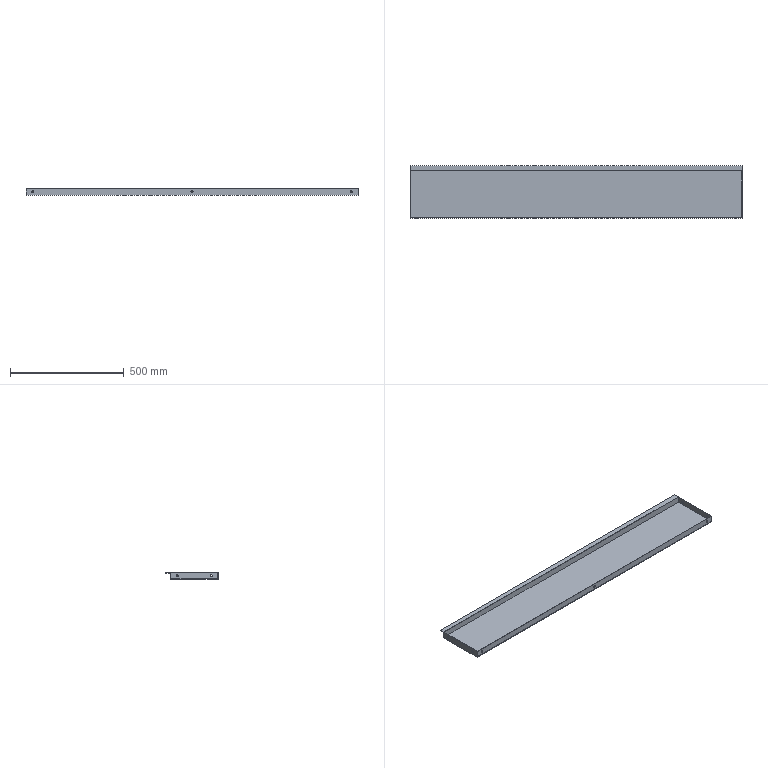Part | SolidWorks | features ICE 3, Extrusion 1, Shell 1 | 1 solid | 27 faces | box 1457 x 230 x 30 mm | volume 855585 mm3 | cylinder 14 | plane 13 | commonest cylinder face diameters 9 x14
STEP:
#1=CARTESIAN_POINT('',(2.,180.,11.5));
#2=VERTEX_POINT('',#1);
#3=CARTESIAN_POINT('',(2.,180.,20.5));
#4=VERTEX_POINT('',#3);
#5=CARTESIAN_POINT('',(2.,180.,16.));
#6=DIRECTION('',(-1.,0.,0.));
#7=DIRECTION('',(0.,0.,-1.));
#8=AXIS2_PLACEMENT_3D('',#5,#6,#7);
#9=CIRCLE('',#8,4.5);
#10=EDGE_CURVE('',#2,#4,#9,.T.);
#11=ORIENTED_EDGE('',*,*,#10,.F.);
#12=CARTESIAN_POINT('',(0.,180.,11.5));
#13=VERTEX_POINT('',#12);
#14=CARTESIAN_POINT('',(1527.,180.,11.5));
#15=DIRECTION('',(-1.,0.,0.));
#16=VECTOR('',#15,1000.);
#17=LINE('',#14,#16);
#18=EDGE_CURVE('',#2,#13,#17,.T.);
#19=ORIENTED_EDGE('',*,*,#18,.T.);
#20=CARTESIAN_POINT('',(0.,180.,20.5));
#21=VERTEX_POINT('',#20);
#22=CARTESIAN_POINT('',(0.,180.,16.));
#23=DIRECTION('',(-1.,0.,0.));
#24=DIRECTION('',(0.,0.,-1.));
#25=AXIS2_PLACEMENT_3D('',#22,#23,#24);
#26=CIRCLE('',#25,4.5);
#27=EDGE_CURVE('',#13,#21,#26,.T.);
#28=ORIENTED_EDGE('',*,*,#27,.T.);
#29=CARTESIAN_POINT('',(1527.,180.,20.5));
#30=DIRECTION('',(-1.,0.,0.));
#31=VECTOR('',#30,1000.);
#32=LINE('',#29,#31);
#33=EDGE_CURVE('',#4,#21,#32,.T.);
#34=ORIENTED_EDGE('',*,*,#33,.F.);
#35=EDGE_LOOP('',(#11,#19,#28,#34));
#36=FACE_OUTER_BOUND('',#35,.T.);
#37=CARTESIAN_POINT('',(1527.,180.,16.));
#38=DIRECTION('',(-1.,0.,0.));
#39=DIRECTION('',(0.,0.,1.));
#40=AXIS2_PLACEMENT_3D('',#37,#38,#39);
#41=CYLINDRICAL_SURFACE('',#40,4.5);
#42=ADVANCED_FACE('',(#36),#41,.F.);
#43=CARTESIAN_POINT('',(1457.,180.,20.5));
#44=VERTEX_POINT('',#43);
#45=CARTESIAN_POINT('',(1457.,180.,11.5));
#46=VERTEX_POINT('',#45);
#47=CARTESIAN_POINT('',(1457.,180.,16.));
#48=DIRECTION('',(1.,0.,0.));
#49=DIRECTION('',(0.,0.,1.));
#50=AXIS2_PLACEMENT_3D('',#47,#48,#49);
#51=CIRCLE('',#50,4.5);
#52=EDGE_CURVE('',#44,#46,#51,.T.);
#53=ORIENTED_EDGE('',*,*,#52,.T.);
#54=CARTESIAN_POINT('',(1455.,180.,11.5));
#55=VERTEX_POINT('',#54);
#56=CARTESIAN_POINT('',(1527.,180.,11.5));
#57=DIRECTION('',(-1.,0.,0.));
#58=VECTOR('',#57,1000.);
#59=LINE('',#56,#58);
#60=EDGE_CURVE('',#46,#55,#59,.T.);
#61=ORIENTED_EDGE('',*,*,#60,.T.);
#62=CARTESIAN_POINT('',(1455.,180.,20.5));
#63=VERTEX_POINT('',#62);
#64=CARTESIAN_POINT('',(1455.,180.,16.));
#65=DIRECTION('',(1.,0.,0.));
#66=DIRECTION('',(0.,0.,1.));
#67=AXIS2_PLACEMENT_3D('',#64,#65,#66);
#68=CIRCLE('',#67,4.5);
#69=EDGE_CURVE('',#63,#55,#68,.T.);
#70=ORIENTED_EDGE('',*,*,#69,.F.);
#71=CARTESIAN_POINT('',(1527.,180.,20.5));
#72=DIRECTION('',(-1.,0.,0.));
#73=VECTOR('',#72,1000.);
#74=LINE('',#71,#73);
#75=EDGE_CURVE('',#44,#63,#74,.T.);
#76=ORIENTED_EDGE('',*,*,#75,.F.);
#77=EDGE_LOOP('',(#53,#61,#70,#76));
#78=FACE_OUTER_BOUND('',#77,.T.);
#79=CARTESIAN_POINT('',(1527.,180.,16.));
#80=DIRECTION('',(-1.,0.,0.));
#81=DIRECTION('',(0.,0.,1.));
#82=AXIS2_PLACEMENT_3D('',#79,#80,#81);
#83=CYLINDRICAL_SURFACE('',#82,4.5);
#84=ADVANCED_FACE('',(#78),#83,.F.);
#85=CARTESIAN_POINT('',(2.,30.,11.5));
#86=VERTEX_POINT('',#85);
#87=CARTESIAN_POINT('',(2.,30.,20.5));
#88=VERTEX_POINT('',#87);
#89=CARTESIAN_POINT('',(2.,30.,16.));
#90=DIRECTION('',(-1.,0.,0.));
#91=DIRECTION('',(0.,0.,-1.));
#92=AXIS2_PLACEMENT_3D('',#89,#90,#91);
#93=CIRCLE('',#92,4.5);
#94=EDGE_CURVE('',#86,#88,#93,.T.);
#95=ORIENTED_EDGE('',*,*,#94,.F.);
#96=CARTESIAN_POINT('',(0.,30.,11.5));
#97=VERTEX_POINT('',#96);
#98=CARTESIAN_POINT('',(1527.,30.,11.5));
#99=DIRECTION('',(-1.,0.,0.));
#100=VECTOR('',#99,1000.);
#101=LINE('',#98,#100);
#102=EDGE_CURVE('',#86,#97,#101,.T.);
#103=ORIENTED_EDGE('',*,*,#102,.T.);
#104=CARTESIAN_POINT('',(0.,30.,20.5));
#105=VERTEX_POINT('',#104);
#106=CARTESIAN_POINT('',(0.,30.,16.));
#107=DIRECTION('',(-1.,0.,0.));
#108=DIRECTION('',(0.,0.,-1.));
#109=AXIS2_PLACEMENT_3D('',#106,#107,#108);
#110=CIRCLE('',#109,4.5);
#111=EDGE_CURVE('',#97,#105,#110,.T.);
#112=ORIENTED_EDGE('',*,*,#111,.T.);
#113=CARTESIAN_POINT('',(1527.,30.,20.5));
#114=DIRECTION('',(-1.,0.,0.));
#115=VECTOR('',#114,1000.);
#116=LINE('',#113,#115);
#117=EDGE_CURVE('',#88,#105,#116,.T.);
#118=ORIENTED_EDGE('',*,*,#117,.F.);
#119=EDGE_LOOP('',(#95,#103,#112,#118));
#120=FACE_OUTER_BOUND('',#119,.T.);
#121=CARTESIAN_POINT('',(1527.,30.,16.));
#122=DIRECTION('',(-1.,0.,0.));
#123=DIRECTION('',(0.,0.,1.));
#124=AXIS2_PLACEMENT_3D('',#121,#122,#123);
#125=CYLINDRICAL_SURFACE('',#124,4.5);
#126=ADVANCED_FACE('',(#120),#125,.F.);
#127=CARTESIAN_POINT('',(1457.,30.,20.5));
#128=VERTEX_POINT('',#127);
#129=CARTESIAN_POINT('',(1457.,30.,11.5));
#130=VERTEX_POINT('',#129);
#131=CARTESIAN_POINT('',(1457.,30.,16.));
#132=DIRECTION('',(1.,0.,0.));
#133=DIRECTION('',(0.,0.,1.));
#134=AXIS2_PLACEMENT_3D('',#131,#132,#133);
#135=CIRCLE('',#134,4.5);
#136=EDGE_CURVE('',#128,#130,#135,.T.);
#137=ORIENTED_EDGE('',*,*,#136,.T.);
#138=CARTESIAN_POINT('',(1455.,30.,11.5));
#139=VERTEX_POINT('',#138);
#140=CARTESIAN_POINT('',(1527.,30.,11.5));
#141=DIRECTION('',(-1.,0.,0.));
#142=VECTOR('',#141,1000.);
#143=LINE('',#140,#142);
#144=EDGE_CURVE('',#130,#139,#143,.T.);
#145=ORIENTED_EDGE('',*,*,#144,.T.);
#146=CARTESIAN_POINT('',(1455.,30.,20.5));
#147=VERTEX_POINT('',#146);
#148=CARTESIAN_POINT('',(1455.,30.,16.));
#149=DIRECTION('',(1.,0.,0.));
#150=DIRECTION('',(0.,0.,1.));
#151=AXIS2_PLACEMENT_3D('',#148,#149,#150);
#152=CIRCLE('',#151,4.5);
#153=EDGE_CURVE('',#147,#139,#152,.T.);
#154=ORIENTED_EDGE('',*,*,#153,.F.);
#155=CARTESIAN_POINT('',(1527.,30.,20.5));
#156=DIRECTION('',(-1.,0.,0.));
#157=VECTOR('',#156,1000.);
#158=LINE('',#155,#157);
#159=EDGE_CURVE('',#128,#147,#158,.T.);
#160=ORIENTED_EDGE('',*,*,#159,.F.);
#161=EDGE_LOOP('',(#137,#145,#154,#160));
#162=FACE_OUTER_BOUND('',#161,.T.);
#163=CARTESIAN_POINT('',(1527.,30.,16.));
#164=DIRECTION('',(-1.,0.,0.));
#165=DIRECTION('',(0.,0.,1.));
#166=AXIS2_PLACEMENT_3D('',#163,#164,#165);
#167=CYLINDRICAL_SURFACE('',#166,4.5);
#168=ADVANCED_FACE('',(#162),#167,.F.);
#169=CARTESIAN_POINT('',(30.,0.,11.5));
#170=VERTEX_POINT('',#169);
#171=CARTESIAN_POINT('',(30.,0.,20.5));
#172=VERTEX_POINT('',#171);
#173=CARTESIAN_POINT('',(30.,0.,16.));
#174=DIRECTION('',(0.,1.,0.));
#175=DIRECTION('',(0.,0.,1.));
#176=AXIS2_PLACEMENT_3D('',#173,#174,#175);
#177=CIRCLE('',#176,4.5);
#178=EDGE_CURVE('',#170,#172,#177,.T.);
#179=ORIENTED_EDGE('',*,*,#178,.F.);
#180=CARTESIAN_POINT('',(30.,2.,11.5));
#181=VERTEX_POINT('',#180);
#182=CARTESIAN_POINT('',(30.,-8.,11.5));
#183=DIRECTION('',(0.,1.,0.));
#184=VECTOR('',#183,1000.);
#185=LINE('',#182,#184);
#186=EDGE_CURVE('',#170,#181,#185,.T.);
#187=ORIENTED_EDGE('',*,*,#186,.T.);
#188=CARTESIAN_POINT('',(30.,2.,20.5));
#189=VERTEX_POINT('',#188);
#190=CARTESIAN_POINT('',(30.,2.,16.));
#191=DIRECTION('',(0.,1.,0.));
#192=DIRECTION('',(0.,0.,1.));
#193=AXIS2_PLACEMENT_3D('',#190,#191,#192);
#194=CIRCLE('',#193,4.5);
#195=EDGE_CURVE('',#181,#189,#194,.T.);
#196=ORIENTED_EDGE('',*,*,#195,.T.);
#197=CARTESIAN_POINT('',(30.,-8.,20.5));
#198=DIRECTION('',(0.,1.,0.));
#199=VECTOR('',#198,1000.);
#200=LINE('',#197,#199);
#201=EDGE_CURVE('',#172,#189,#200,.T.);
#202=ORIENTED_EDGE('',*,*,#201,.F.);
#203=EDGE_LOOP('',(#179,#187,#196,#202));
#204=FACE_OUTER_BOUND('',#203,.T.);
#205=CARTESIAN_POINT('',(30.,-8.,16.));
#206=DIRECTION('',(0.,1.,0.));
#207=DIRECTION('',(0.,0.,1.));
#208=AXIS2_PLACEMENT_3D('',#205,#206,#207);
#209=CYLINDRICAL_SURFACE('',#208,4.5);
#210=ADVANCED_FACE('',(#204),#209,.F.);
#211=CARTESIAN_POINT('',(728.5,0.,11.5));
#212=VERTEX_POINT('',#211);
#213=CARTESIAN_POINT('',(728.5,0.,20.5));
#214=VERTEX_POINT('',#213);
#215=CARTESIAN_POINT('',(728.5,0.,16.));
#216=DIRECTION('',(0.,1.,0.));
#217=DIRECTION('',(0.,0.,1.));
#218=AXIS2_PLACEMENT_3D('',#215,#216,#217);
#219=CIRCLE('',#218,4.5);
#220=EDGE_CURVE('',#212,#214,#219,.T.);
#221=ORIENTED_EDGE('',*,*,#220,.F.);
#222=CARTESIAN_POINT('',(728.5,2.,11.5));
#223=VERTEX_POINT('',#222);
#224=CARTESIAN_POINT('',(728.5,-8.,11.5));
#225=DIRECTION('',(0.,1.,0.));
#226=VECTOR('',#225,1000.);
#227=LINE('',#224,#226);
#228=EDGE_CURVE('',#212,#223,#227,.T.);
#229=ORIENTED_EDGE('',*,*,#228,.T.);
#230=CARTESIAN_POINT('',(728.5,2.,20.5));
#231=VERTEX_POINT('',#230);
#232=CARTESIAN_POINT('',(728.5,2.,16.));
#233=DIRECTION('',(0.,1.,0.));
#234=DIRECTION('',(0.,0.,1.));
#235=AXIS2_PLACEMENT_3D('',#232,#233,#234);
#236=CIRCLE('',#235,4.5);
#237=EDGE_CURVE('',#223,#231,#236,.T.);
#238=ORIENTED_EDGE('',*,*,#237,.T.);
#239=CARTESIAN_POINT('',(728.5,-8.,20.5));
#240=DIRECTION('',(0.,1.,0.));
#241=VECTOR('',#240,1000.);
#242=LINE('',#239,#241);
#243=EDGE_CURVE('',#214,#231,#242,.T.);
#244=ORIENTED_EDGE('',*,*,#243,.F.);
#245=EDGE_LOOP('',(#221,#229,#238,#244));
#246=FACE_OUTER_BOUND('',#245,.T.);
#247=CARTESIAN_POINT('',(728.5,-8.,16.));
#248=DIRECTION('',(0.,1.,0.));
#249=DIRECTION('',(0.,0.,1.));
#250=AXIS2_PLACEMENT_3D('',#247,#248,#249);
#251=CYLINDRICAL_SURFACE('',#250,4.5);
#252=ADVANCED_FACE('',(#246),#251,.F.);
#253=CARTESIAN_POINT('',(1427.,0.,11.5));
#254=VERTEX_POINT('',#253);
#255=CARTESIAN_POINT('',(1427.,0.,20.5));
#256=VERTEX_POINT('',#255);
#257=CARTESIAN_POINT('',(1427.,0.,16.));
#258=DIRECTION('',(0.,1.,0.));
#259=DIRECTION('',(0.,0.,1.));
#260=AXIS2_PLACEMENT_3D('',#257,#258,#259);
#261=CIRCLE('',#260,4.5);
#262=EDGE_CURVE('',#254,#256,#261,.T.);
#263=ORIENTED_EDGE('',*,*,#262,.F.);
#264=CARTESIAN_POINT('',(1427.,2.,11.5));
#265=VERTEX_POINT('',#264);
#266=CARTESIAN_POINT('',(1427.,-8.,11.5));
#267=DIRECTION('',(0.,1.,0.));
#268=VECTOR('',#267,1000.);
#269=LINE('',#266,#268);
#270=EDGE_CURVE('',#254,#265,#269,.T.);
#271=ORIENTED_EDGE('',*,*,#270,.T.);
#272=CARTESIAN_POINT('',(1427.,2.,20.5));
#273=VERTEX_POINT('',#272);
#274=CARTESIAN_POINT('',(1427.,2.,16.));
#275=DIRECTION('',(0.,1.,0.));
#276=DIRECTION('',(0.,0.,1.));
#277=AXIS2_PLACEMENT_3D('',#274,#275,#276);
#278=CIRCLE('',#277,4.5);
#279=EDGE_CURVE('',#265,#273,#278,.T.);
#280=ORIENTED_EDGE('',*,*,#279,.T.);
#281=CARTESIAN_POINT('',(1427.,-8.,20.5));
#282=DIRECTION('',(0.,1.,0.));
#283=VECTOR('',#282,1000.);
#284=LINE('',#281,#283);
#285=EDGE_CURVE('',#256,#273,#284,.T.);
#286=ORIENTED_EDGE('',*,*,#285,.F.);
#287=EDGE_LOOP('',(#263,#271,#280,#286));
#288=FACE_OUTER_BOUND('',#287,.T.);
#289=CARTESIAN_POINT('',(1427.,-8.,16.));
#290=DIRECTION('',(0.,1.,0.));
#291=DIRECTION('',(0.,0.,1.));
#292=AXIS2_PLACEMENT_3D('',#289,#290,#291);
#293=CYLINDRICAL_SURFACE('',#292,4.5);
#294=ADVANCED_FACE('',(#288),#293,.F.);
#295=CARTESIAN_POINT('',(0.,30.,16.));
#296=DIRECTION('',(-1.,0.,0.));
#297=DIRECTION('',(0.,0.,-1.));
#298=AXIS2_PLACEMENT_3D('',#295,#296,#297);
#299=CIRCLE('',#298,4.5);
#300=EDGE_CURVE('',#105,#97,#299,.T.);
#301=ORIENTED_EDGE('',*,*,#300,.F.);
#302=ORIENTED_EDGE('',*,*,#111,.F.);
#303=EDGE_LOOP('',(#301,#302));
#304=FACE_BOUND('',#303,.T.);
#305=CARTESIAN_POINT('',(0.,210.,0.));
#306=VERTEX_POINT('',#305);
#307=CARTESIAN_POINT('',(0.,0.,0.));
#308=VERTEX_POINT('',#307);
#309=CARTESIAN_POINT('',(0.,0.,0.));
#310=DIRECTION('',(0.,-1.,0.));
#311=VECTOR('',#310,1000.);
#312=LINE('',#309,#311);
#313=EDGE_CURVE('',#306,#308,#312,.T.);
#314=ORIENTED_EDGE('',*,*,#313,.T.);
#315=CARTESIAN_POINT('',(0.,0.,30.));
#316=VERTEX_POINT('',#315);
#317=CARTESIAN_POINT('',(0.,0.,30.));
#318=DIRECTION('',(0.,0.,-1.));
#319=VECTOR('',#318,1000.);
#320=LINE('',#317,#319);
#321=EDGE_CURVE('',#316,#308,#320,.T.);
#322=ORIENTED_EDGE('',*,*,#321,.F.);
#323=CARTESIAN_POINT('',(0.,230.,30.));
#324=VERTEX_POINT('',#323);
#325=CARTESIAN_POINT('',(0.,0.,30.));
#326=DIRECTION('',(0.,-1.,0.));
#327=VECTOR('',#326,1000.);
#328=LINE('',#325,#327);
#329=EDGE_CURVE('',#324,#316,#328,.T.);
#330=ORIENTED_EDGE('',*,*,#329,.F.);
#331=CARTESIAN_POINT('',(0.,230.,28.));
#332=VERTEX_POINT('',#331);
#333=CARTESIAN_POINT('',(0.,230.,28.));
#334=DIRECTION('',(0.,0.,1.));
#335=VECTOR('',#334,1000.);
#336=LINE('',#333,#335);
#337=EDGE_CURVE('',#332,#324,#336,.T.);
#338=ORIENTED_EDGE('',*,*,#337,.F.);
#339=CARTESIAN_POINT('',(0.,210.,28.));
#340=VERTEX_POINT('',#339);
#341=CARTESIAN_POINT('',(0.,230.,28.));
#342=DIRECTION('',(0.,-1.,0.));
#343=VECTOR('',#342,1000.);
#344=LINE('',#341,#343);
#345=EDGE_CURVE('',#332,#340,#344,.T.);
#346=ORIENTED_EDGE('',*,*,#345,.T.);
#347=CARTESIAN_POINT('',(0.,210.,30.));
#348=DIRECTION('',(0.,0.,-1.));
#349=VECTOR('',#348,1000.);
#350=LINE('',#347,#349);
#351=EDGE_CURVE('',#340,#306,#350,.T.);
#352=ORIENTED_EDGE('',*,*,#351,.T.);
#353=EDGE_LOOP('',(#314,#322,#330,#338,#346,#352));
#354=FACE_OUTER_BOUND('',#353,.T.);
#355=CARTESIAN_POINT('',(0.,180.,16.));
#356=DIRECTION('',(-1.,0.,0.));
#357=DIRECTION('',(0.,0.,-1.));
#358=AXIS2_PLACEMENT_3D('',#355,#356,#357);
#359=CIRCLE('',#358,4.5);
#360=EDGE_CURVE('',#21,#13,#359,.T.);
#361=ORIENTED_EDGE('',*,*,#360,.F.);
#362=ORIENTED_EDGE('',*,*,#27,.F.);
#363=EDGE_LOOP('',(#361,#362));
#364=FACE_BOUND('',#363,.T.);
#365=CARTESIAN_POINT('',(0.,0.,30.));
#366=DIRECTION('',(1.,0.,0.));
#367=DIRECTION('',(0.,0.,-1.));
#368=AXIS2_PLACEMENT_3D('',#365,#366,#367);
#369=PLANE('',#368);
#370=ADVANCED_FACE('',(#304,#354,#364),#369,.F.);
#371=ORIENTED_EDGE('',*,*,#136,.F.);
#372=CARTESIAN_POINT('',(1457.,30.,16.));
#373=DIRECTION('',(1.,0.,0.));
#374=DIRECTION('',(0.,0.,1.));
#375=AXIS2_PLACEMENT_3D('',#372,#373,#374);
#376=CIRCLE('',#375,4.5);
#377=EDGE_CURVE('',#130,#128,#376,.T.);
#378=ORIENTED_EDGE('',*,*,#377,.F.);
#379=EDGE_LOOP('',(#371,#378));
#380=FACE_BOUND('',#379,.T.);
#381=CARTESIAN_POINT('',(1457.,0.,0.));
#382=VERTEX_POINT('',#381);
#383=CARTESIAN_POINT('',(1457.,210.,0.));
#384=VERTEX_POINT('',#383);
#385=CARTESIAN_POINT('',(1457.,0.,0.));
#386=DIRECTION('',(0.,1.,0.));
#387=VECTOR('',#386,1000.);
#388=LINE('',#385,#387);
#389=EDGE_CURVE('',#382,#384,#388,.T.);
#390=ORIENTED_EDGE('',*,*,#389,.T.);
#391=CARTESIAN_POINT('',(1457.,210.,28.));
#392=VERTEX_POINT('',#391);
#393=CARTESIAN_POINT('',(1457.,210.,30.));
#394=DIRECTION('',(0.,0.,-1.));
#395=VECTOR('',#394,1000.);
#396=LINE('',#393,#395);
#397=EDGE_CURVE('',#392,#384,#396,.T.);
#398=ORIENTED_EDGE('',*,*,#397,.F.);
#399=CARTESIAN_POINT('',(1457.,230.,28.));
#400=VERTEX_POINT('',#399);
#401=CARTESIAN_POINT('',(1457.,210.,28.));
#402=DIRECTION('',(0.,1.,0.));
#403=VECTOR('',#402,1000.);
#404=LINE('',#401,#403);
#405=EDGE_CURVE('',#392,#400,#404,.T.);
#406=ORIENTED_EDGE('',*,*,#405,.T.);
#407=CARTESIAN_POINT('',(1457.,230.,30.));
#408=VERTEX_POINT('',#407);
#409=CARTESIAN_POINT('',(1457.,230.,28.));
#410=DIRECTION('',(0.,0.,1.));
#411=VECTOR('',#410,1000.);
#412=LINE('',#409,#411);
#413=EDGE_CURVE('',#400,#408,#412,.T.);
#414=ORIENTED_EDGE('',*,*,#413,.T.);
#415=CARTESIAN_POINT('',(1457.,0.,30.));
#416=VERTEX_POINT('',#415);
#417=CARTESIAN_POINT('',(1457.,0.,30.));
#418=DIRECTION('',(0.,1.,0.));
#419=VECTOR('',#418,1000.);
#420=LINE('',#417,#419);
#421=EDGE_CURVE('',#416,#408,#420,.T.);
#422=ORIENTED_EDGE('',*,*,#421,.F.);
#423=CARTESIAN_POINT('',(1457.,0.,30.));
#424=DIRECTION('',(0.,0.,-1.));
#425=VECTOR('',#424,1000.);
#426=LINE('',#423,#425);
#427=EDGE_CURVE('',#416,#382,#426,.T.);
#428=ORIENTED_EDGE('',*,*,#427,.T.);
#429=EDGE_LOOP('',(#390,#398,#406,#414,#422,#428));
#430=FACE_OUTER_BOUND('',#429,.T.);
#431=ORIENTED_EDGE('',*,*,#52,.F.);
#432=CARTESIAN_POINT('',(1457.,180.,16.));
#433=DIRECTION('',(1.,0.,0.));
#434=DIRECTION('',(0.,0.,1.));
#435=AXIS2_PLACEMENT_3D('',#432,#433,#434);
#436=CIRCLE('',#435,4.5);
#437=EDGE_CURVE('',#46,#44,#436,.T.);
#438=ORIENTED_EDGE('',*,*,#437,.F.);
#439=EDGE_LOOP('',(#431,#438));
#440=FACE_BOUND('',#439,.T.);
#441=CARTESIAN_POINT('',(1457.,0.,30.));
#442=DIRECTION('',(-1.,0.,0.));
#443=DIRECTION('',(0.,0.,1.));
#444=AXIS2_PLACEMENT_3D('',#441,#442,#443);
#445=PLANE('',#444);
#446=ADVANCED_FACE('',(#380,#430,#440),#445,.F.);
#447=CARTESIAN_POINT('',(2.,30.,16.));
#448=DIRECTION('',(-1.,0.,0.));
#449=DIRECTION('',(0.,0.,-1.));
#450=AXIS2_PLACEMENT_3D('',#447,#448,#449);
#451=CIRCLE('',#450,4.5);
#452=EDGE_CURVE('',#88,#86,#451,.T.);
#453=ORIENTED_EDGE('',*,*,#452,.T.);
#454=ORIENTED_EDGE('',*,*,#94,.T.);
#455=EDGE_LOOP('',(#453,#454));
#456=FACE_BOUND('',#455,.T.);
#457=CARTESIAN_POINT('',(2.,208.,2.));
#458=VERTEX_POINT('',#457);
#459=CARTESIAN_POINT('',(2.,2.,2.));
#460=VERTEX_POINT('',#459);
#461=CARTESIAN_POINT('',(2.,210.,2.));
#462=DIRECTION('',(0.,-1.,0.));
#463=VECTOR('',#462,1000.);
#464=LINE('',#461,#463);
#465=EDGE_CURVE('',#458,#460,#464,.T.);
#466=ORIENTED_EDGE('',*,*,#465,.F.);
#467=CARTESIAN_POINT('',(2.,208.,30.));
#468=VERTEX_POINT('',#467);
#469=CARTESIAN_POINT('',(2.,208.,30.));
#470=DIRECTION('',(0.,0.,-1.));
#471=VECTOR('',#470,1000.);
#472=LINE('',#469,#471);
#473=EDGE_CURVE('',#468,#458,#472,.T.);
#474=ORIENTED_EDGE('',*,*,#473,.F.);
#475=CARTESIAN_POINT('',(2.,2.,30.));
#476=VERTEX_POINT('',#475);
#477=CARTESIAN_POINT('',(2.,210.,30.));
#478=DIRECTION('',(0.,-1.,0.));
#479=VECTOR('',#478,1000.);
#480=LINE('',#477,#479);
#481=EDGE_CURVE('',#468,#476,#480,.T.);
#482=ORIENTED_EDGE('',*,*,#481,.T.);
#483=CARTESIAN_POINT('',(2.,2.,30.));
#484=DIRECTION('',(0.,0.,-1.));
#485=VECTOR('',#484,1000.);
#486=LINE('',#483,#485);
#487=EDGE_CURVE('',#476,#460,#486,.T.);
#488=ORIENTED_EDGE('',*,*,#487,.T.);
#489=EDGE_LOOP('',(#466,#474,#482,#488));
#490=FACE_OUTER_BOUND('',#489,.T.);
#491=CARTESIAN_POINT('',(2.,180.,16.));
#492=DIRECTION('',(-1.,0.,0.));
#493=DIRECTION('',(0.,0.,-1.));
#494=AXIS2_PLACEMENT_3D('',#491,#492,#493);
#495=CIRCLE('',#494,4.5);
#496=EDGE_CURVE('',#4,#2,#495,.T.);
#497=ORIENTED_EDGE('',*,*,#496,.T.);
#498=ORIENTED_EDGE('',*,*,#10,.T.);
#499=EDGE_LOOP('',(#497,#498));
#500=FACE_BOUND('',#499,.T.);
#501=CARTESIAN_POINT('',(2.,0.,30.));
#502=DIRECTION('',(1.,0.,0.));
#503=DIRECTION('',(0.,0.,-1.));
#504=AXIS2_PLACEMENT_3D('',#501,#502,#503);
#505=PLANE('',#504);
#506=ADVANCED_FACE('',(#456,#490,#500),#505,.T.);
#507=ORIENTED_EDGE('',*,*,#153,.T.);
#508=CARTESIAN_POINT('',(1455.,30.,16.));
#509=DIRECTION('',(1.,0.,0.));
#510=DIRECTION('',(0.,0.,1.));
#511=AXIS2_PLACEMENT_3D('',#508,#509,#510);
#512=CIRCLE('',#511,4.5);
#513=EDGE_CURVE('',#139,#147,#512,.T.);
#514=ORIENTED_EDGE('',*,*,#513,.T.);
#515=EDGE_LOOP('',(#507,#514));
#516=FACE_BOUND('',#515,.T.);
#517=CARTESIAN_POINT('',(1455.,2.,2.));
#518=VERTEX_POINT('',#517);
#519=CARTESIAN_POINT('',(1455.,208.,2.));
#520=VERTEX_POINT('',#519);
#521=CARTESIAN_POINT('',(1455.,210.,2.));
#522=DIRECTION('',(0.,1.,0.));
#523=VECTOR('',#522,1000.);
#524=LINE('',#521,#523);
#525=EDGE_CURVE('',#518,#520,#524,.T.);
#526=ORIENTED_EDGE('',*,*,#525,.F.);
#527=CARTESIAN_POINT('',(1455.,2.,30.));
#528=VERTEX_POINT('',#527);
#529=CARTESIAN_POINT('',(1455.,2.,30.));
#530=DIRECTION('',(0.,0.,-1.));
#531=VECTOR('',#530,1000.);
#532=LINE('',#529,#531);
#533=EDGE_CURVE('',#528,#518,#532,.T.);
#534=ORIENTED_EDGE('',*,*,#533,.F.);
#535=CARTESIAN_POINT('',(1455.,208.,30.));
#536=VERTEX_POINT('',#535);
#537=CARTESIAN_POINT('',(1455.,210.,30.));
#538=DIRECTION('',(0.,1.,0.));
#539=VECTOR('',#538,1000.);
#540=LINE('',#537,#539);
#541=EDGE_CURVE('',#528,#536,#540,.T.);
#542=ORIENTED_EDGE('',*,*,#541,.T.);
#543=CARTESIAN_POINT('',(1455.,208.,30.));
#544=DIRECTION('',(0.,0.,-1.));
#545=VECTOR('',#544,1000.);
#546=LINE('',#543,#545);
#547=EDGE_CURVE('',#536,#520,#546,.T.);
#548=ORIENTED_EDGE('',*,*,#547,.T.);
#549=EDGE_LOOP('',(#526,#534,#542,#548));
#550=FACE_OUTER_BOUND('',#549,.T.);
#551=ORIENTED_EDGE('',*,*,#69,.T.);
#552=CARTESIAN_POINT('',(1455.,180.,16.));
#553=DIRECTION('',(1.,0.,0.));
#554=DIRECTION('',(0.,0.,1.));
#555=AXIS2_PLACEMENT_3D('',#552,#553,#554);
#556=CIRCLE('',#555,4.5);
#557=EDGE_CURVE('',#55,#63,#556,.T.);
#558=ORIENTED_EDGE('',*,*,#557,.T.);
#559=EDGE_LOOP('',(#551,#558));
#560=FACE_BOUND('',#559,.T.);
#561=CARTESIAN_POINT('',(1455.,0.,30.));
#562=DIRECTION('',(-1.,0.,0.));
#563=DIRECTION('',(0.,0.,1.));
#564=AXIS2_PLACEMENT_3D('',#561,#562,#563);
#565=PLANE('',#564);
#566=ADVANCED_FACE('',(#516,#550,#560),#565,.T.);
#567=ORIENTED_EDGE('',*,*,#329,.T.);
#568=CARTESIAN_POINT('',(0.,0.,30.));
#569=DIRECTION('',(1.,0.,0.));
#570=VECTOR('',#569,1000.);
#571=LINE('',#568,#570);
#572=EDGE_CURVE('',#316,#416,#571,.T.);
#573=ORIENTED_EDGE('',*,*,#572,.T.);
#574=ORIENTED_EDGE('',*,*,#421,.T.);
#575=CARTESIAN_POINT('',(0.,230.,30.));
#576=DIRECTION('',(-1.,0.,0.));
#577=VECTOR('',#576,1000.);
#578=LINE('',#575,#577);
#579=EDGE_CURVE('',#408,#324,#578,.T.);
#580=ORIENTED_EDGE('',*,*,#579,.T.);
#581=EDGE_LOOP('',(#567,#573,#574,#580));
#582=FACE_OUTER_BOUND('',#581,.T.);
#583=ORIENTED_EDGE('',*,*,#481,.F.);
#584=CARTESIAN_POINT('',(0.,208.,30.));
#585=DIRECTION('',(-1.,0.,0.));
#586=VECTOR('',#585,1000.);
#587=LINE('',#584,#586);
#588=EDGE_CURVE('',#536,#468,#587,.T.);
#589=ORIENTED_EDGE('',*,*,#588,.F.);
#590=ORIENTED_EDGE('',*,*,#541,.F.);
#591=CARTESIAN_POINT('',(0.,2.,30.));
#592=DIRECTION('',(1.,0.,0.));
#593=VECTOR('',#592,1000.);
#594=LINE('',#591,#593);
#595=EDGE_CURVE('',#476,#528,#594,.T.);
#596=ORIENTED_EDGE('',*,*,#595,.F.);
#597=EDGE_LOOP('',(#583,#589,#590,#596));
#598=FACE_BOUND('',#597,.T.);
#599=CARTESIAN_POINT('',(0.,210.,30.));
#600=DIRECTION('',(0.,0.,-1.));
#601=DIRECTION('',(-1.,0.,0.));
#602=AXIS2_PLACEMENT_3D('',#599,#600,#601);
#603=PLANE('',#602);
#604=ADVANCED_FACE('',(#582,#598),#603,.F.);
#605=CARTESIAN_POINT('',(30.,0.,16.));
#606=DIRECTION('',(0.,1.,0.));
#607=DIRECTION('',(0.,0.,1.));
#608=AXIS2_PLACEMENT_3D('',#605,#606,#607);
#609=CIRCLE('',#608,4.5);
#610=EDGE_CURVE('',#172,#170,#609,.T.);
#611=ORIENTED_EDGE('',*,*,#610,.T.);
#612=ORIENTED_EDGE('',*,*,#178,.T.);
#613=EDGE_LOOP('',(#611,#612));
#614=FACE_BOUND('',#613,.T.);
#615=CARTESIAN_POINT('',(728.5,0.,16.));
#616=DIRECTION('',(0.,1.,0.));
#617=DIRECTION('',(0.,0.,1.));
#618=AXIS2_PLACEMENT_3D('',#615,#616,#617);
#619=CIRCLE('',#618,4.5);
#620=EDGE_CURVE('',#214,#212,#619,.T.);
#621=ORIENTED_EDGE('',*,*,#620,.T.);
#622=ORIENTED_EDGE('',*,*,#220,.T.);
#623=EDGE_LOOP('',(#621,#622));
#624=FACE_BOUND('',#623,.T.);
#625=CARTESIAN_POINT('',(1427.,0.,16.));
#626=DIRECTION('',(0.,1.,0.));
#627=DIRECTION('',(0.,0.,1.));
#628=AXIS2_PLACEMENT_3D('',#625,#626,#627);
#629=CIRCLE('',#628,4.5);
#630=EDGE_CURVE('',#256,#254,#629,.T.);
#631=ORIENTED_EDGE('',*,*,#630,.T.);
#632=ORIENTED_EDGE('',*,*,#262,.T.);
#633=EDGE_LOOP('',(#631,#632));
#634=FACE_BOUND('',#633,.T.);
#635=CARTESIAN_POINT('',(0.,0.,0.));
#636=DIRECTION('',(1.,0.,0.));
#637=VECTOR('',#636,1000.);
#638=LINE('',#635,#637);
#639=EDGE_CURVE('',#308,#382,#638,.T.);
#640=ORIENTED_EDGE('',*,*,#639,.T.);
#641=ORIENTED_EDGE('',*,*,#427,.F.);
#642=ORIENTED_EDGE('',*,*,#572,.F.);
#643=ORIENTED_EDGE('',*,*,#321,.T.);
#644=EDGE_LOOP('',(#640,#641,#642,#643));
#645=FACE_OUTER_BOUND('',#644,.T.);
#646=CARTESIAN_POINT('',(0.,0.,30.));
#647=DIRECTION('',(0.,1.,0.));
#648=DIRECTION('',(0.,0.,1.));
#649=AXIS2_PLACEMENT_3D('',#646,#647,#648);
#650=PLANE('',#649);
#651=ADVANCED_FACE('',(#614,#624,#634,#645),#650,.F.);
#652=ORIENTED_EDGE('',*,*,#351,.F.);
#653=CARTESIAN_POINT('',(0.,210.,28.));
#654=DIRECTION('',(1.,0.,0.));
#655=VECTOR('',#654,1000.);
#656=LINE('',#653,#655);
#657=EDGE_CURVE('',#340,#392,#656,.T.);
#658=ORIENTED_EDGE('',*,*,#657,.T.);
#659=ORIENTED_EDGE('',*,*,#397,.T.);
#660=CARTESIAN_POINT('',(0.,210.,0.));
#661=DIRECTION('',(-1.,0.,0.));
#662=VECTOR('',#661,1000.);
#663=LINE('',#660,#662);
#664=EDGE_CURVE('',#384,#306,#663,.T.);
#665=ORIENTED_EDGE('',*,*,#664,.T.);
#666=EDGE_LOOP('',(#652,#658,#659,#665));
#667=FACE_OUTER_BOUND('',#666,.T.);
#668=CARTESIAN_POINT('',(0.,210.,30.));
#669=DIRECTION('',(0.,-1.,0.));
#670=DIRECTION('',(0.,0.,-1.));
#671=AXIS2_PLACEMENT_3D('',#668,#669,#670);
#672=PLANE('',#671);
#673=ADVANCED_FACE('',(#667),#672,.F.);
#674=ORIENTED_EDGE('',*,*,#313,.F.);
#675=ORIENTED_EDGE('',*,*,#664,.F.);
#676=ORIENTED_EDGE('',*,*,#389,.F.);
#677=ORIENTED_EDGE('',*,*,#639,.F.);
#678=EDGE_LOOP('',(#674,#675,#676,#677));
#679=FACE_OUTER_BOUND('',#678,.T.);
#680=CARTESIAN_POINT('',(0.,210.,0.));
#681=DIRECTION('',(0.,0.,-1.));
#682=DIRECTION('',(-1.,0.,0.));
#683=AXIS2_PLACEMENT_3D('',#680,#681,#682);
#684=PLANE('',#683);
#685=ADVANCED_FACE('',(#679),#684,.T.);
#686=CARTESIAN_POINT('',(30.,2.,16.));
#687=DIRECTION('',(0.,1.,0.));
#688=DIRECTION('',(0.,0.,1.));
#689=AXIS2_PLACEMENT_3D('',#686,#687,#688);
#690=CIRCLE('',#689,4.5);
#691=EDGE_CURVE('',#189,#181,#690,.T.);
#692=ORIENTED_EDGE('',*,*,#691,.F.);
#693=ORIENTED_EDGE('',*,*,#195,.F.);
#694=EDGE_LOOP('',(#692,#693));
#695=FACE_BOUND('',#694,.T.);
#696=CARTESIAN_POINT('',(728.5,2.,16.));
#697=DIRECTION('',(0.,1.,0.));
#698=DIRECTION('',(0.,0.,1.));
#699=AXIS2_PLACEMENT_3D('',#696,#697,#698);
#700=CIRCLE('',#699,4.5);
#701=EDGE_CURVE('',#231,#223,#700,.T.);
#702=ORIENTED_EDGE('',*,*,#701,.F.);
#703=ORIENTED_EDGE('',*,*,#237,.F.);
#704=EDGE_LOOP('',(#702,#703));
#705=FACE_BOUND('',#704,.T.);
#706=CARTESIAN_POINT('',(1427.,2.,16.));
#707=DIRECTION('',(0.,1.,0.));
#708=DIRECTION('',(0.,0.,1.));
#709=AXIS2_PLACEMENT_3D('',#706,#707,#708);
#710=CIRCLE('',#709,4.5);
#711=EDGE_CURVE('',#273,#265,#710,.T.);
#712=ORIENTED_EDGE('',*,*,#711,.F.);
#713=ORIENTED_EDGE('',*,*,#279,.F.);
#714=EDGE_LOOP('',(#712,#713));
#715=FACE_BOUND('',#714,.T.);
#716=CARTESIAN_POINT('',(0.,2.,2.));
#717=DIRECTION('',(1.,0.,0.));
#718=VECTOR('',#717,1000.);
#719=LINE('',#716,#718);
#720=EDGE_CURVE('',#460,#518,#719,.T.);
#721=ORIENTED_EDGE('',*,*,#720,.F.);
#722=ORIENTED_EDGE('',*,*,#487,.F.);
#723=ORIENTED_EDGE('',*,*,#595,.T.);
#724=ORIENTED_EDGE('',*,*,#533,.T.);
#725=EDGE_LOOP('',(#721,#722,#723,#724));
#726=FACE_OUTER_BOUND('',#725,.T.);
#727=CARTESIAN_POINT('',(0.,2.,30.));
#728=DIRECTION('',(0.,1.,0.));
#729=DIRECTION('',(0.,0.,1.));
#730=AXIS2_PLACEMENT_3D('',#727,#728,#729);
#731=PLANE('',#730);
#732=ADVANCED_FACE('',(#695,#705,#715,#726),#731,.T.);
#733=CARTESIAN_POINT('',(0.,208.,2.));
#734=DIRECTION('',(-1.,0.,0.));
#735=VECTOR('',#734,1000.);
#736=LINE('',#733,#735);
#737=EDGE_CURVE('',#520,#458,#736,.T.);
#738=ORIENTED_EDGE('',*,*,#737,.F.);
#739=ORIENTED_EDGE('',*,*,#547,.F.);
#740=ORIENTED_EDGE('',*,*,#588,.T.);
#741=ORIENTED_EDGE('',*,*,#473,.T.);
#742=EDGE_LOOP('',(#738,#739,#740,#741));
#743=FACE_OUTER_BOUND('',#742,.T.);
#744=CARTESIAN_POINT('',(0.,208.,30.));
#745=DIRECTION('',(0.,-1.,0.));
#746=DIRECTION('',(0.,0.,-1.));
#747=AXIS2_PLACEMENT_3D('',#744,#745,#746);
#748=PLANE('',#747);
#749=ADVANCED_FACE('',(#743),#748,.T.);
#750=ORIENTED_EDGE('',*,*,#465,.T.);
#751=ORIENTED_EDGE('',*,*,#720,.T.);
#752=ORIENTED_EDGE('',*,*,#525,.T.);
#753=ORIENTED_EDGE('',*,*,#737,.T.);
#754=EDGE_LOOP('',(#750,#751,#752,#753));
#755=FACE_OUTER_BOUND('',#754,.T.);
#756=CARTESIAN_POINT('',(0.,210.,2.));
#757=DIRECTION('',(0.,0.,-1.));
#758=DIRECTION('',(-1.,0.,0.));
#759=AXIS2_PLACEMENT_3D('',#756,#757,#758);
#760=PLANE('',#759);
#761=ADVANCED_FACE('',(#755),#760,.F.);
#762=ORIENTED_EDGE('',*,*,#579,.F.);
#763=ORIENTED_EDGE('',*,*,#413,.F.);
#764=CARTESIAN_POINT('',(0.,230.,28.));
#765=DIRECTION('',(-1.,0.,0.));
#766=VECTOR('',#765,1000.);
#767=LINE('',#764,#766);
#768=EDGE_CURVE('',#400,#332,#767,.T.);
#769=ORIENTED_EDGE('',*,*,#768,.T.);
#770=ORIENTED_EDGE('',*,*,#337,.T.);
#771=EDGE_LOOP('',(#762,#763,#769,#770));
#772=FACE_OUTER_BOUND('',#771,.T.);
#773=CARTESIAN_POINT('',(0.,230.,28.));
#774=DIRECTION('',(0.,1.,0.));
#775=DIRECTION('',(-1.,0.,0.));
#776=AXIS2_PLACEMENT_3D('',#773,#774,#775);
#777=PLANE('',#776);
#778=ADVANCED_FACE('',(#772),#777,.T.);
#779=ORIENTED_EDGE('',*,*,#345,.F.);
#780=ORIENTED_EDGE('',*,*,#768,.F.);
#781=ORIENTED_EDGE('',*,*,#405,.F.);
#782=ORIENTED_EDGE('',*,*,#657,.F.);
#783=EDGE_LOOP('',(#779,#780,#781,#782));
#784=FACE_OUTER_BOUND('',#783,.T.);
#785=CARTESIAN_POINT('',(0.,210.,28.));
#786=DIRECTION('',(0.,0.,1.));
#787=DIRECTION('',(1.,0.,0.));
#788=AXIS2_PLACEMENT_3D('',#785,#786,#787);
#789=PLANE('',#788);
#790=ADVANCED_FACE('',(#784),#789,.F.);
#791=ORIENTED_EDGE('',*,*,#270,.F.);
#792=ORIENTED_EDGE('',*,*,#630,.F.);
#793=ORIENTED_EDGE('',*,*,#285,.T.);
#794=ORIENTED_EDGE('',*,*,#711,.T.);
#795=EDGE_LOOP('',(#791,#792,#793,#794));
#796=FACE_OUTER_BOUND('',#795,.T.);
#797=CARTESIAN_POINT('',(1427.,-8.,16.));
#798=DIRECTION('',(0.,1.,0.));
#799=DIRECTION('',(0.,0.,1.));
#800=AXIS2_PLACEMENT_3D('',#797,#798,#799);
#801=CYLINDRICAL_SURFACE('',#800,4.5);
#802=ADVANCED_FACE('',(#796),#801,.F.);
#803=ORIENTED_EDGE('',*,*,#228,.F.);
#804=ORIENTED_EDGE('',*,*,#620,.F.);
#805=ORIENTED_EDGE('',*,*,#243,.T.);
#806=ORIENTED_EDGE('',*,*,#701,.T.);
#807=EDGE_LOOP('',(#803,#804,#805,#806));
#808=FACE_OUTER_BOUND('',#807,.T.);
#809=CARTESIAN_POINT('',(728.5,-8.,16.));
#810=DIRECTION('',(0.,1.,0.));
#811=DIRECTION('',(0.,0.,1.));
#812=AXIS2_PLACEMENT_3D('',#809,#810,#811);
#813=CYLINDRICAL_SURFACE('',#812,4.5);
#814=ADVANCED_FACE('',(#808),#813,.F.);
#815=ORIENTED_EDGE('',*,*,#186,.F.);
#816=ORIENTED_EDGE('',*,*,#610,.F.);
#817=ORIENTED_EDGE('',*,*,#201,.T.);
#818=ORIENTED_EDGE('',*,*,#691,.T.);
#819=EDGE_LOOP('',(#815,#816,#817,#818));
#820=FACE_OUTER_BOUND('',#819,.T.);
#821=CARTESIAN_POINT('',(30.,-8.,16.));
#822=DIRECTION('',(0.,1.,0.));
#823=DIRECTION('',(0.,0.,1.));
#824=AXIS2_PLACEMENT_3D('',#821,#822,#823);
#825=CYLINDRICAL_SURFACE('',#824,4.5);
#826=ADVANCED_FACE('',(#820),#825,.F.);
#827=ORIENTED_EDGE('',*,*,#144,.F.);
#828=ORIENTED_EDGE('',*,*,#377,.T.);
#829=ORIENTED_EDGE('',*,*,#159,.T.);
#830=ORIENTED_EDGE('',*,*,#513,.F.);
#831=EDGE_LOOP('',(#827,#828,#829,#830));
#832=FACE_OUTER_BOUND('',#831,.T.);
#833=CARTESIAN_POINT('',(1527.,30.,16.));
#834=DIRECTION('',(-1.,0.,0.));
#835=DIRECTION('',(0.,0.,1.));
#836=AXIS2_PLACEMENT_3D('',#833,#834,#835);
#837=CYLINDRICAL_SURFACE('',#836,4.5);
#838=ADVANCED_FACE('',(#832),#837,.F.);
#839=ORIENTED_EDGE('',*,*,#102,.F.);
#840=ORIENTED_EDGE('',*,*,#452,.F.);
#841=ORIENTED_EDGE('',*,*,#117,.T.);
#842=ORIENTED_EDGE('',*,*,#300,.T.);
#843=EDGE_LOOP('',(#839,#840,#841,#842));
#844=FACE_OUTER_BOUND('',#843,.T.);
#845=CARTESIAN_POINT('',(1527.,30.,16.));
#846=DIRECTION('',(-1.,0.,0.));
#847=DIRECTION('',(0.,0.,1.));
#848=AXIS2_PLACEMENT_3D('',#845,#846,#847);
#849=CYLINDRICAL_SURFACE('',#848,4.5);
#850=ADVANCED_FACE('',(#844),#849,.F.);
#851=ORIENTED_EDGE('',*,*,#60,.F.);
#852=ORIENTED_EDGE('',*,*,#437,.T.);
#853=ORIENTED_EDGE('',*,*,#75,.T.);
#854=ORIENTED_EDGE('',*,*,#557,.F.);
#855=EDGE_LOOP('',(#851,#852,#853,#854));
#856=FACE_OUTER_BOUND('',#855,.T.);
#857=CARTESIAN_POINT('',(1527.,180.,16.));
#858=DIRECTION('',(-1.,0.,0.));
#859=DIRECTION('',(0.,0.,1.));
#860=AXIS2_PLACEMENT_3D('',#857,#858,#859);
#861=CYLINDRICAL_SURFACE('',#860,4.5);
#862=ADVANCED_FACE('',(#856),#861,.F.);
#863=ORIENTED_EDGE('',*,*,#18,.F.);
#864=ORIENTED_EDGE('',*,*,#496,.F.);
#865=ORIENTED_EDGE('',*,*,#33,.T.);
#866=ORIENTED_EDGE('',*,*,#360,.T.);
#867=EDGE_LOOP('',(#863,#864,#865,#866));
#868=FACE_OUTER_BOUND('',#867,.T.);
#869=CARTESIAN_POINT('',(1527.,180.,16.));
#870=DIRECTION('',(-1.,0.,0.));
#871=DIRECTION('',(0.,0.,1.));
#872=AXIS2_PLACEMENT_3D('',#869,#870,#871);
#873=CYLINDRICAL_SURFACE('',#872,4.5);
#874=ADVANCED_FACE('',(#868),#873,.F.);
#875=CLOSED_SHELL('',(#42,#84,#126,#168,#210,#252,#294,#370,#446,#506,#566,#604,#651,#673,#685,#732,#749,#761,#778,#790,#802,#814,#826,#838,#850,#862,#874));
#876=MANIFOLD_SOLID_BREP('',#875);
#877=CARTESIAN_POINT('',(0.,0.,0.));
#878=DIRECTION('',(0.,0.,1.));
#879=DIRECTION('',(1.,0.,0.));
#880=AXIS2_PLACEMENT_3D('',#877,#878,#879);
#881=(LENGTH_UNIT()NAMED_UNIT(*)SI_UNIT(.MILLI.,.METRE.));
#882=UNCERTAINTY_MEASURE_WITH_UNIT(LENGTH_MEASURE(0.00001),#881,'','');
#883=(NAMED_UNIT(*)PLANE_ANGLE_UNIT()SI_UNIT($,.RADIAN.));
#884=(NAMED_UNIT(*)SI_UNIT($,.STERADIAN.)SOLID_ANGLE_UNIT());
#885=(GEOMETRIC_REPRESENTATION_CONTEXT(3)GLOBAL_UNCERTAINTY_ASSIGNED_CONTEXT((#882))GLOBAL_UNIT_ASSIGNED_CONTEXT((#881,#883,#884))REPRESENTATION_CONTEXT('',''));
#886=ADVANCED_BREP_SHAPE_REPRESENTATION('',(#876,#880),#885);